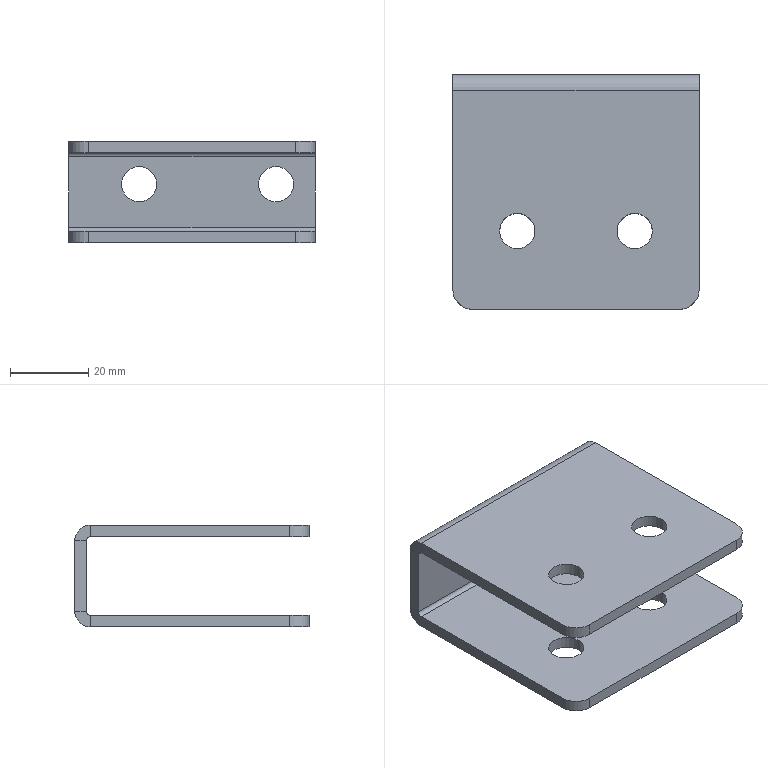Part | STEP file | 5090504 | 1 solid | 32 faces | box 63 x 60 x 26 mm | volume 24845 mm3 | plane 18 | cylinder 14 | commonest cylinder face diameters 9 x6 10 x4 2 x2 8 x2